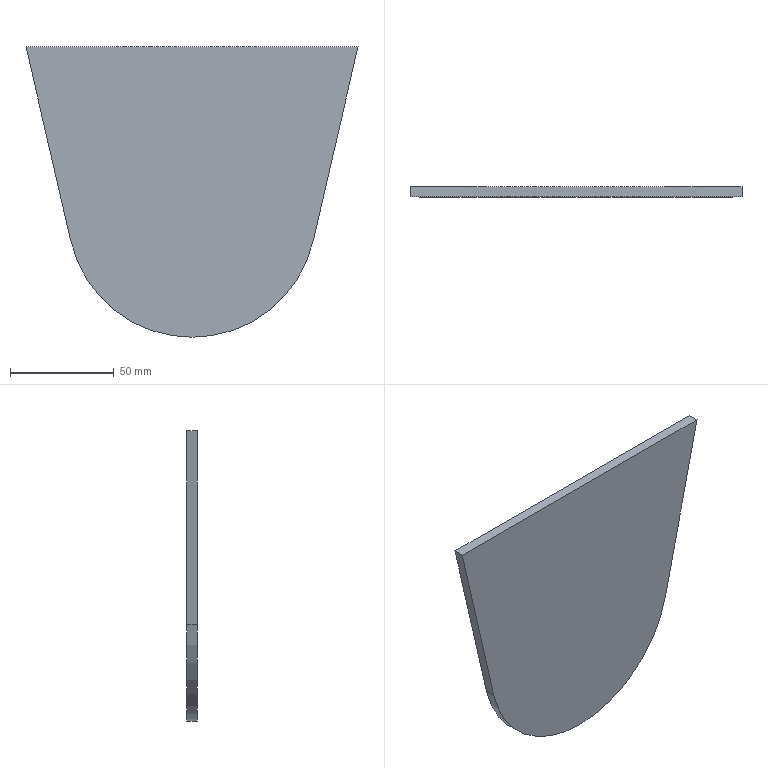Part | SolidWorks | features Extrusion 1 | 1 solid | 7 faces | box 160 x 5 x 140 mm | volume 84974 mm3 | plane 5 | cylinder 2 | commonest cylinder face diameters 120 x2
STEP:
#1=CARTESIAN_POINT('',(0.,5.,-60.));
#2=VERTEX_POINT('',#1);
#3=CARTESIAN_POINT('',(-58.469,5.,-13.469));
#4=VERTEX_POINT('',#3);
#5=CARTESIAN_POINT('',(0.,5.,0.));
#6=DIRECTION('',(0.,1.,0.));
#7=DIRECTION('',(0.,0.,1.));
#8=AXIS2_PLACEMENT_3D('',#5,#6,#7);
#9=CIRCLE('',#8,60.);
#10=EDGE_CURVE('',#2,#4,#9,.T.);
#11=ORIENTED_EDGE('',*,*,#10,.F.);
#12=CARTESIAN_POINT('',(0.,0.,-60.));
#13=VERTEX_POINT('',#12);
#14=CARTESIAN_POINT('',(0.,5.,-60.));
#15=DIRECTION('',(0.,-1.,0.));
#16=VECTOR('',#15,1000.);
#17=LINE('',#14,#16);
#18=EDGE_CURVE('',#2,#13,#17,.T.);
#19=ORIENTED_EDGE('',*,*,#18,.T.);
#20=CARTESIAN_POINT('',(-58.469,0.,-13.469));
#21=VERTEX_POINT('',#20);
#22=CARTESIAN_POINT('',(0.,0.,0.));
#23=DIRECTION('',(0.,1.,0.));
#24=DIRECTION('',(0.,0.,1.));
#25=AXIS2_PLACEMENT_3D('',#22,#23,#24);
#26=CIRCLE('',#25,60.);
#27=EDGE_CURVE('',#13,#21,#26,.T.);
#28=ORIENTED_EDGE('',*,*,#27,.T.);
#29=CARTESIAN_POINT('',(-58.469,5.,-13.469));
#30=DIRECTION('',(0.,-1.,0.));
#31=VECTOR('',#30,1000.);
#32=LINE('',#29,#31);
#33=EDGE_CURVE('',#4,#21,#32,.T.);
#34=ORIENTED_EDGE('',*,*,#33,.F.);
#35=EDGE_LOOP('',(#11,#19,#28,#34));
#36=FACE_OUTER_BOUND('',#35,.T.);
#37=CARTESIAN_POINT('',(0.,5.,0.));
#38=DIRECTION('',(0.,-1.,0.));
#39=DIRECTION('',(0.,0.,-1.));
#40=AXIS2_PLACEMENT_3D('',#37,#38,#39);
#41=CYLINDRICAL_SURFACE('',#40,60.);
#42=ADVANCED_FACE('',(#36),#41,.T.);
#43=CARTESIAN_POINT('',(80.,0.,80.));
#44=VERTEX_POINT('',#43);
#45=CARTESIAN_POINT('',(58.469,0.,-13.469));
#46=VERTEX_POINT('',#45);
#47=CARTESIAN_POINT('',(80.,0.,80.));
#48=DIRECTION('',(-0.2245,0.,-0.9745));
#49=VECTOR('',#48,1000.);
#50=LINE('',#47,#49);
#51=EDGE_CURVE('',#44,#46,#50,.T.);
#52=ORIENTED_EDGE('',*,*,#51,.T.);
#53=CARTESIAN_POINT('',(58.469,5.,-13.469));
#54=VERTEX_POINT('',#53);
#55=CARTESIAN_POINT('',(58.469,5.,-13.469));
#56=DIRECTION('',(0.,-1.,0.));
#57=VECTOR('',#56,1000.);
#58=LINE('',#55,#57);
#59=EDGE_CURVE('',#54,#46,#58,.T.);
#60=ORIENTED_EDGE('',*,*,#59,.F.);
#61=CARTESIAN_POINT('',(80.,5.,80.));
#62=VERTEX_POINT('',#61);
#63=CARTESIAN_POINT('',(80.,5.,80.));
#64=DIRECTION('',(-0.2245,0.,-0.9745));
#65=VECTOR('',#64,1000.);
#66=LINE('',#63,#65);
#67=EDGE_CURVE('',#62,#54,#66,.T.);
#68=ORIENTED_EDGE('',*,*,#67,.F.);
#69=CARTESIAN_POINT('',(80.,5.,80.));
#70=DIRECTION('',(0.,-1.,0.));
#71=VECTOR('',#70,1000.);
#72=LINE('',#69,#71);
#73=EDGE_CURVE('',#62,#44,#72,.T.);
#74=ORIENTED_EDGE('',*,*,#73,.T.);
#75=EDGE_LOOP('',(#52,#60,#68,#74));
#76=FACE_OUTER_BOUND('',#75,.T.);
#77=CARTESIAN_POINT('',(80.,5.,80.));
#78=DIRECTION('',(-0.9745,0.,0.2245));
#79=DIRECTION('',(0.2245,0.,0.9745));
#80=AXIS2_PLACEMENT_3D('',#77,#78,#79);
#81=PLANE('',#80);
#82=ADVANCED_FACE('',(#76),#81,.F.);
#83=ORIENTED_EDGE('',*,*,#18,.F.);
#84=CARTESIAN_POINT('',(0.,5.,0.));
#85=DIRECTION('',(0.,1.,0.));
#86=DIRECTION('',(0.,0.,1.));
#87=AXIS2_PLACEMENT_3D('',#84,#85,#86);
#88=CIRCLE('',#87,60.);
#89=EDGE_CURVE('',#54,#2,#88,.T.);
#90=ORIENTED_EDGE('',*,*,#89,.F.);
#91=ORIENTED_EDGE('',*,*,#59,.T.);
#92=CARTESIAN_POINT('',(0.,0.,0.));
#93=DIRECTION('',(0.,1.,0.));
#94=DIRECTION('',(0.,0.,1.));
#95=AXIS2_PLACEMENT_3D('',#92,#93,#94);
#96=CIRCLE('',#95,60.);
#97=EDGE_CURVE('',#46,#13,#96,.T.);
#98=ORIENTED_EDGE('',*,*,#97,.T.);
#99=EDGE_LOOP('',(#83,#90,#91,#98));
#100=FACE_OUTER_BOUND('',#99,.T.);
#101=CARTESIAN_POINT('',(0.,5.,0.));
#102=DIRECTION('',(0.,-1.,0.));
#103=DIRECTION('',(0.,0.,-1.));
#104=AXIS2_PLACEMENT_3D('',#101,#102,#103);
#105=CYLINDRICAL_SURFACE('',#104,60.);
#106=ADVANCED_FACE('',(#100),#105,.T.);
#107=CARTESIAN_POINT('',(-80.,0.,80.));
#108=VERTEX_POINT('',#107);
#109=CARTESIAN_POINT('',(-80.,0.,80.));
#110=DIRECTION('',(-0.2245,0.,0.9745));
#111=VECTOR('',#110,1000.);
#112=LINE('',#109,#111);
#113=EDGE_CURVE('',#21,#108,#112,.T.);
#114=ORIENTED_EDGE('',*,*,#113,.T.);
#115=CARTESIAN_POINT('',(-80.,5.,80.));
#116=VERTEX_POINT('',#115);
#117=CARTESIAN_POINT('',(-80.,5.,80.));
#118=DIRECTION('',(0.,-1.,0.));
#119=VECTOR('',#118,1000.);
#120=LINE('',#117,#119);
#121=EDGE_CURVE('',#116,#108,#120,.T.);
#122=ORIENTED_EDGE('',*,*,#121,.F.);
#123=CARTESIAN_POINT('',(-80.,5.,80.));
#124=DIRECTION('',(-0.2245,0.,0.9745));
#125=VECTOR('',#124,1000.);
#126=LINE('',#123,#125);
#127=EDGE_CURVE('',#4,#116,#126,.T.);
#128=ORIENTED_EDGE('',*,*,#127,.F.);
#129=ORIENTED_EDGE('',*,*,#33,.T.);
#130=EDGE_LOOP('',(#114,#122,#128,#129));
#131=FACE_OUTER_BOUND('',#130,.T.);
#132=CARTESIAN_POINT('',(-80.,5.,80.));
#133=DIRECTION('',(0.9745,0.,0.2245));
#134=DIRECTION('',(0.2245,0.,-0.9745));
#135=AXIS2_PLACEMENT_3D('',#132,#133,#134);
#136=PLANE('',#135);
#137=ADVANCED_FACE('',(#131),#136,.F.);
#138=CARTESIAN_POINT('',(80.,0.,80.));
#139=DIRECTION('',(1.,0.,0.));
#140=VECTOR('',#139,1000.);
#141=LINE('',#138,#140);
#142=EDGE_CURVE('',#108,#44,#141,.T.);
#143=ORIENTED_EDGE('',*,*,#142,.T.);
#144=ORIENTED_EDGE('',*,*,#73,.F.);
#145=CARTESIAN_POINT('',(80.,5.,80.));
#146=DIRECTION('',(1.,0.,0.));
#147=VECTOR('',#146,1000.);
#148=LINE('',#145,#147);
#149=EDGE_CURVE('',#116,#62,#148,.T.);
#150=ORIENTED_EDGE('',*,*,#149,.F.);
#151=ORIENTED_EDGE('',*,*,#121,.T.);
#152=EDGE_LOOP('',(#143,#144,#150,#151));
#153=FACE_OUTER_BOUND('',#152,.T.);
#154=CARTESIAN_POINT('',(80.,5.,80.));
#155=DIRECTION('',(0.,0.,-1.));
#156=DIRECTION('',(-1.,0.,0.));
#157=AXIS2_PLACEMENT_3D('',#154,#155,#156);
#158=PLANE('',#157);
#159=ADVANCED_FACE('',(#153),#158,.F.);
#160=ORIENTED_EDGE('',*,*,#67,.T.);
#161=ORIENTED_EDGE('',*,*,#89,.T.);
#162=ORIENTED_EDGE('',*,*,#10,.T.);
#163=ORIENTED_EDGE('',*,*,#127,.T.);
#164=ORIENTED_EDGE('',*,*,#149,.T.);
#165=EDGE_LOOP('',(#160,#161,#162,#163,#164));
#166=FACE_OUTER_BOUND('',#165,.T.);
#167=CARTESIAN_POINT('',(0.,5.,0.));
#168=DIRECTION('',(0.,1.,0.));
#169=DIRECTION('',(0.,0.,1.));
#170=AXIS2_PLACEMENT_3D('',#167,#168,#169);
#171=PLANE('',#170);
#172=ADVANCED_FACE('',(#166),#171,.T.);
#173=ORIENTED_EDGE('',*,*,#51,.F.);
#174=ORIENTED_EDGE('',*,*,#142,.F.);
#175=ORIENTED_EDGE('',*,*,#113,.F.);
#176=ORIENTED_EDGE('',*,*,#27,.F.);
#177=ORIENTED_EDGE('',*,*,#97,.F.);
#178=EDGE_LOOP('',(#173,#174,#175,#176,#177));
#179=FACE_OUTER_BOUND('',#178,.T.);
#180=CARTESIAN_POINT('',(0.,0.,0.));
#181=DIRECTION('',(0.,1.,0.));
#182=DIRECTION('',(0.,0.,1.));
#183=AXIS2_PLACEMENT_3D('',#180,#181,#182);
#184=PLANE('',#183);
#185=ADVANCED_FACE('',(#179),#184,.F.);
#186=CLOSED_SHELL('',(#42,#82,#106,#137,#159,#172,#185));
#187=MANIFOLD_SOLID_BREP('',#186);
#188=CARTESIAN_POINT('',(0.,0.,0.));
#189=DIRECTION('',(0.,0.,1.));
#190=DIRECTION('',(1.,0.,0.));
#191=AXIS2_PLACEMENT_3D('',#188,#189,#190);
#192=(LENGTH_UNIT()NAMED_UNIT(*)SI_UNIT(.MILLI.,.METRE.));
#193=UNCERTAINTY_MEASURE_WITH_UNIT(LENGTH_MEASURE(0.00001),#192,'','');
#194=(NAMED_UNIT(*)PLANE_ANGLE_UNIT()SI_UNIT($,.RADIAN.));
#195=(NAMED_UNIT(*)SI_UNIT($,.STERADIAN.)SOLID_ANGLE_UNIT());
#196=(GEOMETRIC_REPRESENTATION_CONTEXT(3)GLOBAL_UNCERTAINTY_ASSIGNED_CONTEXT((#193))GLOBAL_UNIT_ASSIGNED_CONTEXT((#192,#194,#195))REPRESENTATION_CONTEXT('',''));
#197=ADVANCED_BREP_SHAPE_REPRESENTATION('',(#187,#191),#196);